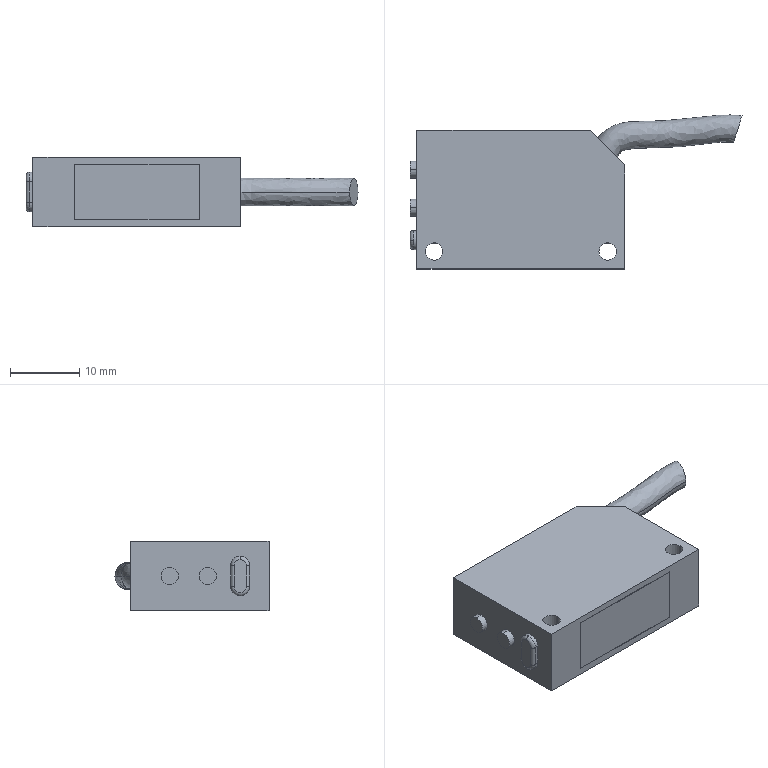Part | STEP file | 501-04-0011 | 1 solid | 36 faces | box 47.887 x 22.217 x 10 mm | volume 6035 mm3 | plane 18 | cylinder 13 | torus 3 | spline 2 | commonest cylinder face diameters 2.5 x8 2.748 x3 1 x2